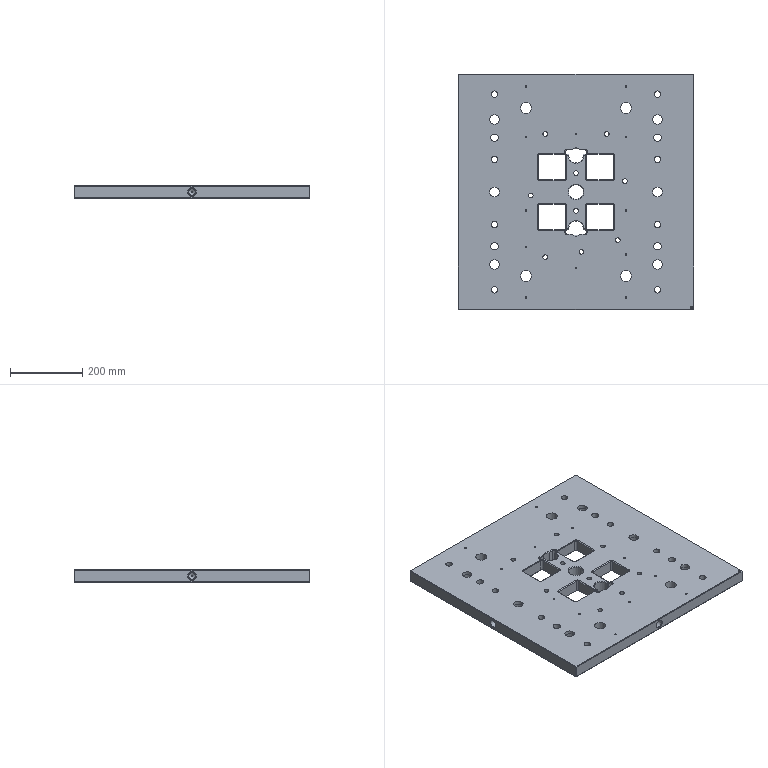Part | STEP file | P011002B004-000 | 1 solid | 629 faces | box 650 x 650 x 35 mm | volume 13284442 mm3 | plane 387 | cylinder 127 | cone 98 | other 17 | commonest cylinder face diameters 20 x17 10 x16 26 x14 4.167 x12 4.983 x12 5 x12